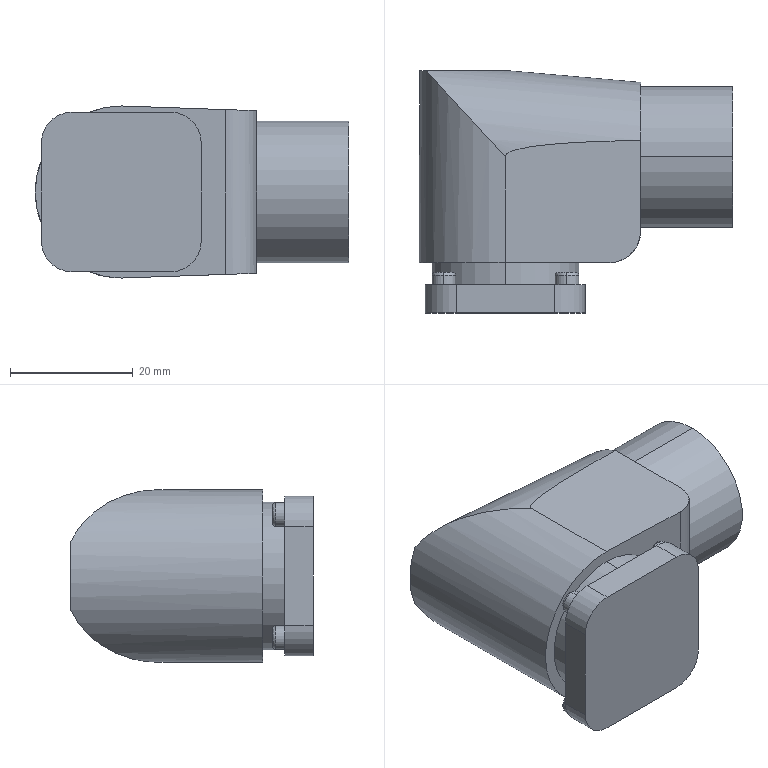Part | STEP file | _BMH070 Signalstecker gerade1 | 1 solid | 83 faces | box 51 x 39.4 x 28 mm | volume 34337 mm3 | cylinder 46 | plane 29 | spline 8 | commonest cylinder face diameters 1 x24 3.8 x8 10 x5 28 x3 19 x2 23 x2